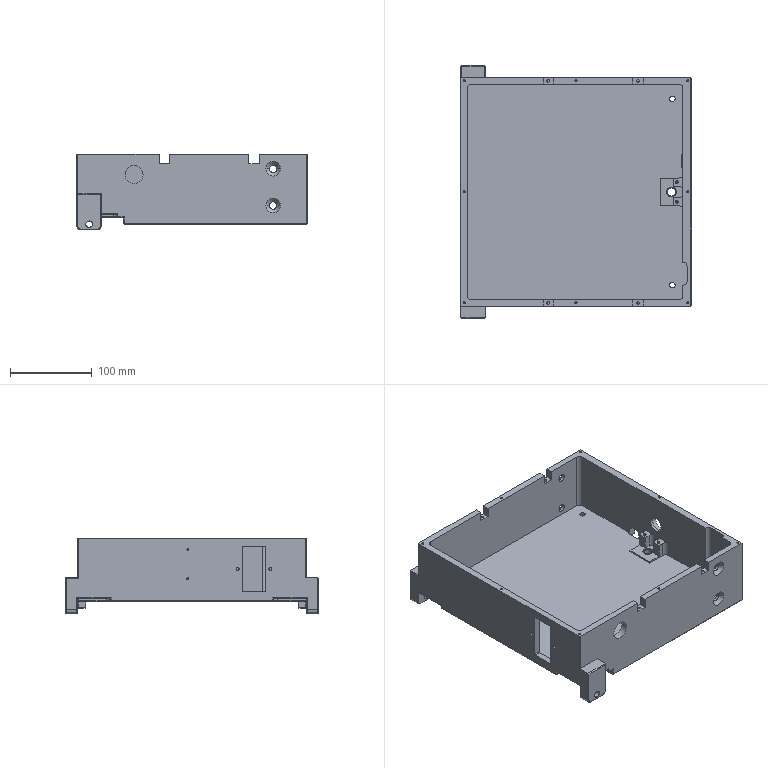NC program | Mastercam | posted with a generic post
Lines 36208 to 38289 of 104433, first 1964 of 2082 lines:
(10 FEM |TOOL - 10|DIA. OFF. - 10|LEN. - 10|TOOL DIA. - 10.)
N3176 T10 M6
N3178 G0 G54 G90 X-125. Y35.15 C0. B0. S7000 M3
N3180 G43 H10 Z50.
N3182 Z1.
N3184 G1 Z-.7 F600.
N3186 X-132. F3000.
N3188 X-140.
N3190 X-147.
N3192 Z-1.4 F600.
N3194 X-140. F3000.
N3196 X-132.
N3198 X-125.
N3200 Z-2.1 F600.
N3202 X-132. F3000.
N3204 X-140.
N3206 X-147.
N3208 Z-2.8 F600.
N3210 X-140. F3000.
N3212 X-132.
N3214 X-125.
N3216 Z-3.5 F600.
N3218 X-132. F3000.
N3220 X-140.
N3222 X-147.
N3224 Z-4.2 F600.
N3226 X-140. F3000.
N3228 X-132.
N3230 X-125.
N3232 Z-4.9 F600.
N3234 X-132. F3000.
N3236 X-140.
N3238 X-147.
N3240 Z-5.6 F600.
N3242 X-140. F3000.
N3244 X-132.
N3246 X-125.
N3248 Z-6.3 F600.
N3250 X-132. F3000.
N3252 X-140.
N3254 X-147.
N3256 Z-7. F600.
N3258 X-140. F3000.
N3260 X-132.
N3262 X-125.
N3264 Z-7.7 F600.
N3266 X-132. F3000.
N3268 X-140.
N3270 X-147.
N3272 Z-8.4 F600.
N3274 X-140. F3000.
N3276 X-132.
N3278 X-125.
N3280 Z-9.1 F600.
N3282 X-132. F3000.
N3284 X-140.
N3286 X-147.
N3288 Z-9.8 F600.
N3290 X-140. F3000.
N3292 X-132.
N3294 X-125.
N3296 Z-10.5 F600.
N3298 X-132. F3000.
N3300 X-140.
N3302 X-147.
N3304 Z-11.2 F600.
N3306 X-140. F3000.
N3308 X-132.
N3310 X-125.
N3312 Z-11.9 F600.
N3314 X-132. F3000.
N3316 X-140.
N3318 X-147.
N3320 G0 Z50.
N3322 Y32.85
N3324 Z1.
N3326 G1 Z-.7 F600.
N3328 X-140. F3000.
N3330 X-132.
N3332 X-125.
N3334 Z-1.4 F600.
N3336 X-132. F3000.
N3338 X-140.
N3340 X-147.
N3342 Z-2.1 F600.
N3344 X-140. F3000.
N3346 X-132.
N3348 X-125.
N3350 Z-2.8 F600.
N3352 X-132. F3000.
N3354 X-140.
N3356 X-147.
N3358 Z-3.5 F600.
N3360 X-140. F3000.
N3362 X-132.
N3364 X-125.
N3366 Z-4.2 F600.
N3368 X-132. F3000.
N3370 X-140.
N3372 X-147.
N3374 Z-4.9 F600.
N3376 X-140. F3000.
N3378 X-132.
N3380 X-125.
N3382 Z-5.6 F600.
N3384 X-132. F3000.
N3386 X-140.
N3388 X-147.
N3390 Z-6.3 F600.
N3392 X-140. F3000.
N3394 X-132.
N3396 X-125.
N3398 Z-7. F600.
N3400 X-132. F3000.
N3402 X-140.
N3404 X-147.
N3406 Z-7.7 F600.
N3408 X-140. F3000.
N3410 X-132.
N3412 X-125.
N3414 Z-8.4 F600.
N3416 X-132. F3000.
N3418 X-140.
N3420 X-147.
N3422 Z-9.1 F600.
N3424 X-140. F3000.
N3426 X-132.
N3428 X-125.
N3430 Z-9.8 F600.
N3432 X-132. F3000.
N3434 X-140.
N3436 X-147.
N3438 Z-10.5 F600.
N3440 X-140. F3000.
N3442 X-132.
N3444 X-125.
N3446 Z-11.2 F600.
N3448 X-132. F3000.
N3450 X-140.
N3452 X-147.
N3454 Z-11.9 F600.
N3456 X-140. F3000.
N3458 X-132.
N3460 X-125.
N3462 G0 Z50.
N3464 Y-74.85
N3466 Z1.
N3468 G1 Z-.7 F600.
N3470 X-132. F3000.
N3472 X-140.
N3474 X-147.
N3476 Z-1.4 F600.
N3478 X-140. F3000.
N3480 X-132.
N3482 X-125.
N3484 Z-2.1 F600.
N3486 X-132. F3000.
N3488 X-140.
N3490 X-147.
N3492 Z-2.8 F600.
N3494 X-140. F3000.
N3496 X-132.
N3498 X-125.
N3500 Z-3.5 F600.
N3502 X-132. F3000.
N3504 X-140.
N3506 X-147.
N3508 Z-4.2 F600.
N3510 X-140. F3000.
N3512 X-132.
N3514 X-125.
N3516 Z-4.9 F600.
N3518 X-132. F3000.
N3520 X-140.
N3522 X-147.
N3524 Z-5.6 F600.
N3526 X-140. F3000.
N3528 X-132.
N3530 X-125.
N3532 Z-6.3 F600.
N3534 X-132. F3000.
N3536 X-140.
N3538 X-147.
N3540 Z-7. F600.
N3542 X-140. F3000.
N3544 X-132.
N3546 X-125.
N3548 Z-7.7 F600.
N3550 X-132. F3000.
N3552 X-140.
N3554 X-147.
N3556 Z-8.4 F600.
N3558 X-140. F3000.
N3560 X-132.
N3562 X-125.
N3564 Z-9.1 F600.
N3566 X-132. F3000.
N3568 X-140.
N3570 X-147.
N3572 Z-9.8 F600.
N3574 X-140. F3000.
N3576 X-132.
N3578 X-125.
N3580 Z-10.5 F600.
N3582 X-132. F3000.
N3584 X-140.
N3586 X-147.
N3588 Z-11.2 F600.
N3590 X-140. F3000.
N3592 X-132.
N3594 X-125.
N3596 Z-11.9 F600.
N3598 X-132. F3000.
N3600 X-140.
N3602 X-147.
N3604 G0 Z50.
N3606 Y-77.15
N3608 Z1.
N3610 G1 Z-.7 F600.
N3612 X-140. F3000.
N3614 X-132.
N3616 X-125.
N3618 Z-1.4 F600.
N3620 X-132. F3000.
N3622 X-140.
N3624 X-147.
N3626 Z-2.1 F600.
N3628 X-140. F3000.
N3630 X-132.
N3632 X-125.
N3634 Z-2.8 F600.
N3636 X-132. F3000.
N3638 X-140.
N3640 X-147.
N3642 Z-3.5 F600.
N3644 X-140. F3000.
N3646 X-132.
N3648 X-125.
N3650 Z-4.2 F600.
N3652 X-132. F3000.
N3654 X-140.
N3656 X-147.
N3658 Z-4.9 F600.
N3660 X-140. F3000.
N3662 X-132.
N3664 X-125.
N3666 Z-5.6 F600.
N3668 X-132. F3000.
N3670 X-140.
N3672 X-147.
N3674 Z-6.3 F600.
N3676 X-140. F3000.
N3678 X-132.
N3680 X-125.
N3682 Z-7. F600.
N3684 X-132. F3000.
N3686 X-140.
N3688 X-147.
N3690 Z-7.7 F600.
N3692 X-140. F3000.
N3694 X-132.
N3696 X-125.
N3698 Z-8.4 F600.
N3700 X-132. F3000.
N3702 X-140.
N3704 X-147.
N3706 Z-9.1 F600.
N3708 X-140. F3000.
N3710 X-132.
N3712 X-125.
N3714 Z-9.8 F600.
N3716 X-132. F3000.
N3718 X-140.
N3720 X-147.
N3722 Z-10.5 F600.
N3724 X-140. F3000.
N3726 X-132.
N3728 X-125.
N3730 Z-11.2 F600.
N3732 X-132. F3000.
N3734 X-140.
N3736 X-147.
N3738 Z-11.9 F600.
N3740 X-140. F3000.
N3742 X-132.
N3744 X-125.
N3746 G0 Z50.
N3748 X147. Y-74.85
N3750 Z1.
N3752 G1 Z-.7 F600.
N3754 X140. F3000.
N3756 X132.
N3758 X125.
N3760 Z-1.4 F600.
N3762 X132. F3000.
N3764 X140.
N3766 X147.
N3768 Z-2.1 F600.
N3770 X140. F3000.
N3772 X132.
N3774 X125.
N3776 Z-2.8 F600.
N3778 X132. F3000.
N3780 X140.
N3782 X147.
N3784 Z-3.5 F600.
N3786 X140. F3000.
N3788 X132.
N3790 X125.
N3792 Z-4.2 F600.
N3794 X132. F3000.
N3796 X140.
N3798 X147.
N3800 Z-4.9 F600.
N3802 X140. F3000.
N3804 X132.
N3806 X125.
N3808 Z-5.6 F600.
N3810 X132. F3000.
N3812 X140.
N3814 X147.
N3816 Z-6.3 F600.
N3818 X140. F3000.
N3820 X132.
N3822 X125.
N3824 Z-7. F600.
N3826 X132. F3000.
N3828 X140.
N3830 X147.
N3832 Z-7.7 F600.
N3834 X140. F3000.
N3836 X132.
N3838 X125.
N3840 Z-8.4 F600.
N3842 X132. F3000.
N3844 X140.
N3846 X147.
N3848 Z-9.1 F600.
N3850 X140. F3000.
N3852 X132.
N3854 X125.
N3856 Z-9.8 F600.
N3858 X132. F3000.
N3860 X140.
N3862 X147.
N3864 Z-10.5 F600.
N3866 X140. F3000.
N3868 X132.
N3870 X125.
N3872 Z-11.2 F600.
N3874 X132. F3000.
N3876 X140.
N3878 X147.
N3880 Z-11.9 F600.
N3882 X140. F3000.
N3884 X132.
N3886 X125.
N3888 G0 Z50.
N3890 Y-77.15
N3892 Z1.
N3894 G1 Z-.7 F600.
N3896 X132. F3000.
N3898 X140.
N3900 X147.
N3902 Z-1.4 F600.
N3904 X140. F3000.
N3906 X132.
N3908 X125.
N3910 Z-2.1 F600.
N3912 X132. F3000.
N3914 X140.
N3916 X147.
N3918 Z-2.8 F600.
N3920 X140. F3000.
N3922 X132.
N3924 X125.
N3926 Z-3.5 F600.
N3928 X132. F3000.
N3930 X140.
N3932 X147.
N3934 Z-4.2 F600.
N3936 X140. F3000.
N3938 X132.
N3940 X125.
N3942 Z-4.9 F600.
N3944 X132. F3000.
N3946 X140.
N3948 X147.
N3950 Z-5.6 F600.
N3952 X140. F3000.
N3954 X132.
N3956 X125.
N3958 Z-6.3 F600.
N3960 X132. F3000.
N3962 X140.
N3964 X147.
N3966 Z-7. F600.
N3968 X140. F3000.
N3970 X132.
N3972 X125.
N3974 Z-7.7 F600.
N3976 X132. F3000.
N3978 X140.
N3980 X147.
N3982 Z-8.4 F600.
N3984 X140. F3000.
N3986 X132.
N3988 X125.
N3990 Z-9.1 F600.
N3992 X132. F3000.
N3994 X140.
N3996 X147.
N3998 Z-9.8 F600.
N4000 X140. F3000.
N4002 X132.
N4004 X125.
N4006 Z-10.5 F600.
N4008 X132. F3000.
N4010 X140.
N4012 X147.
N4014 Z-11.2 F600.
N4016 X140. F3000.
N4018 X132.
N4020 X125.
N4022 Z-11.9 F600.
N4024 X132. F3000.
N4026 X140.
N4028 X147.
N4030 G0 Z50.
N4032 Y35.15
N4034 Z1.
N4036 G1 Z-.7 F600.
N4038 X140. F3000.
N4040 X132.
N4042 X125.
N4044 Z-1.4 F600.
N4046 X132. F3000.
N4048 X140.
N4050 X147.
N4052 Z-2.1 F600.
N4054 X140. F3000.
N4056 X132.
N4058 X125.
N4060 Z-2.8 F600.
N4062 X132. F3000.
N4064 X140.
N4066 X147.
N4068 Z-3.5 F600.
N4070 X140. F3000.
N4072 X132.
N4074 X125.
N4076 Z-4.2 F600.
N4078 X132. F3000.
N4080 X140.
N4082 X147.
N4084 Z-4.9 F600.
N4086 X140. F3000.
N4088 X132.
N4090 X125.
N4092 Z-5.6 F600.
N4094 X132. F3000.
N4096 X140.
N4098 X147.
N4100 Z-6.3 F600.
N4102 X140. F3000.
N4104 X132.
N4106 X125.
N4108 Z-7. F600.
N4110 X132. F3000.
N4112 X140.
N4114 X147.
N4116 Z-7.7 F600.
N4118 X140. F3000.
N4120 X132.
N4122 X125.
N4124 Z-8.4 F600.
N4126 X132. F3000.
N4128 X140.
N4130 X147.
N4132 Z-9.1 F600.
N4134 X140. F3000.
N4136 X132.
N4138 X125.
N4140 Z-9.8 F600.
N4142 X132. F3000.
N4144 X140.
N4146 X147.
N4148 Z-10.5 F600.
N4150 X140. F3000.
N4152 X132.
N4154 X125.
N4156 Z-11.2 F600.
N4158 X132. F3000.
N4160 X140.
N4162 X147.
N4164 Z-11.9 F600.
N4166 X140. F3000.
N4168 X132.
N4170 X125.
N4172 G0 Z50.
N4174 Y32.85
N4176 Z1.
N4178 G1 Z-.7 F600.
N4180 X132. F3000.
N4182 X140.
N4184 X147.
N4186 Z-1.4 F600.
N4188 X140. F3000.
N4190 X132.
N4192 X125.
N4194 Z-2.1 F600.
N4196 X132. F3000.
N4198 X140.
N4200 X147.
N4202 Z-2.8 F600.
N4204 X140. F3000.
N4206 X132.
N4208 X125.
N4210 Z-3.5 F600.
N4212 X132. F3000.
N4214 X140.
N4216 X147.
N4218 Z-4.2 F600.
N4220 X140. F3000.
N4222 X132.
N4224 X125.
N4226 Z-4.9 F600.
N4228 X132. F3000.
N4230 X140.
N4232 X147.
N4234 Z-5.6 F600.
N4236 X140. F3000.
N4238 X132.
N4240 X125.
N4242 Z-6.3 F600.
N4244 X132. F3000.
N4246 X140.
N4248 X147.
N4250 Z-7. F600.
N4252 X140. F3000.
N4254 X132.
N4256 X125.
N4258 Z-7.7 F600.
N4260 X132. F3000.
N4262 X140.
N4264 X147.
N4266 Z-8.4 F600.
N4268 X140. F3000.
N4270 X132.
N4272 X125.
N4274 Z-9.1 F600.
N4276 X132. F3000.
N4278 X140.
N4280 X147.
N4282 Z-9.8 F600.
N4284 X140. F3000.
N4286 X132.
N4288 X125.
N4290 Z-10.5 F600.
N4292 X132. F3000.
N4294 X140.
N4296 X147.
N4298 Z-11.2 F600.
N4300 X140. F3000.
N4302 X132.
N4304 X125.
N4306 Z-11.9 F600.
N4308 X132. F3000.
N4310 X140.
N4312 X147.
N4314 G0 Z50.
N4316 X-125. Y35.26
N4318 Z1.
N4320 G1 Z-12. F600.
N4322 X-132. F1000.
N4324 X-140.
N4326 X-147.
N4328 G0 Z50.
N4330 Y32.74
N4332 Z1.
N4334 G1 Z-12. F600.
N4336 X-140. F1000.
N4338 X-132.
N4340 X-125.
N4342 G0 Z50.
N4344 Y-74.74
N4346 Z1.
N4348 G1 Z-12. F600.
N4350 X-132. F1000.
N4352 X-140.
N4354 X-147.
N4356 G0 Z50.
N4358 Y-77.26
N4360 Z1.
N4362 G1 Z-12. F600.
N4364 X-140. F1000.
N4366 X-132.
N4368 X-125.
N4370 G0 Z50.
N4372 X147. Y-74.74
N4374 Z1.
N4376 G1 Z-12. F600.
N4378 X140. F1000.
N4380 X132.
N4382 X125.
N4384 G0 Z50.
N4386 Y-77.26
N4388 Z1.
N4390 G1 Z-12. F600.
N4392 X132. F1000.
N4394 X140.
N4396 X147.
N4398 G0 Z50.
N4400 Y35.26
N4402 Z1.
N4404 G1 Z-12. F600.
N4406 X140. F1000.
N4408 X132.
N4410 X125.
N4412 G0 Z50.
N4414 Y32.74
N4416 Z1.
N4418 G1 Z-12. F600.
N4420 X132. F1000.
N4422 X140.
N4424 X147.
N4426 G0 Z50.
N4428 M5
N4430 G0 G28 G91 Z0.
N4432 G28
N4434 M01
N4436 G0 G17 G40 G80 G90 G94 G98
N4438 G0 G28 G91 Z0.
(20 FEM |TOOL - 20|DIA. OFF. - 20|LEN. - 20|TOOL DIA. - 20.)
N4440 T20 M6
N4442 G0 G54 G90 X155.627 Y-138.656 C0. B0. S4000 M3
N4444 G43 H20 Z50.
N4446 Z1.
N4448 G1 Z-24. F600.
N4450 X147.142 Y-147.142 F2000.
N4452 X146.142 Y-148.142
N4454 G2 X139. Y-151.1 I-7.142 J7.142
N4456 G1 X-139.
N4458 G2 X-146.142 Y-148.142 J10.1
N4460 G1 X-147.142 Y-147.142
N4462 G2 X-150.1 Y-140. I7.142 J7.142
N4464 G1 Y140.
N4466 G2 X-147.142 Y147.142 I10.1
N4468 G1 X-146.142 Y148.142
N4470 G2 X-139. Y151.1 I7.142 J-7.142
N4472 G1 X139.
N4474 G2 X146.142 Y148.142 J-10.1
N4476 G1 X147.142 Y147.142
N4478 G2 X150.1 Y140. I-7.142 J-7.142
N4480 G1 Y-140.
N4482 G2 X147.142 Y-147.142 I-10.1
N4484 G1 X146.788 Y-147.495
N4486 X137.596 Y-156.688
N4488 G0 Z50.
N4490 X155.556 Y-138.586
N4492 Z1.
N4494 G1 Z-24. F600.
N4496 X147.071 Y-147.071 F2000.
N4498 X146.071 Y-148.071
N4500 G2 X139. Y-151. I-7.071 J7.071
N4502 G1 X-139.
N4504 G2 X-146.071 Y-148.071 J10.
N4506 G1 X-147.071 Y-147.071
N4508 G2 X-150. Y-140. I7.071 J7.071
N4510 G1 Y140.
N4512 G2 X-147.071 Y147.071 I10.
N4514 G1 X-146.071 Y148.071
N4516 G2 X-139. Y151. I7.071 J-7.071
N4518 G1 X139.
N4520 G2 X146.071 Y148.071 J-10.
N4522 G1 X147.071 Y147.071
N4524 G2 X150. Y140. I-7.071 J-7.071
N4526 G1 Y-140.
N4528 G2 X147.071 Y-147.071 I-10.
N4530 G1 X146.718 Y-147.425
N4532 X137.525 Y-156.617
N4534 G0 Z50.
N4536 X155.627 Y-138.656
N4538 Z-23.
N4540 G1 Z-48. F600.
N4542 X147.142 Y-147.142 F2000.
N4544 X146.142 Y-148.142
N4546 G2 X139. Y-151.1 I-7.142 J7.142
N4548 G1 X-139.
N4550 G2 X-146.142 Y-148.142 J10.1
N4552 G1 X-147.142 Y-147.142
N4554 G2 X-150.1 Y-140. I7.142 J7.142
N4556 G1 Y140.
N4558 G2 X-147.142 Y147.142 I10.1
N4560 G1 X-146.142 Y148.142
N4562 G2 X-139. Y151.1 I7.142 J-7.142
N4564 G1 X139.
N4566 G2 X146.142 Y148.142 J-10.1
N4568 G1 X147.142 Y147.142
N4570 G2 X150.1 Y140. I-7.142 J-7.142
N4572 G1 Y-140.
N4574 G2 X147.142 Y-147.142 I-10.1
N4576 G1 X146.788 Y-147.495
N4578 X137.596 Y-156.688
N4580 G0 Z50.
N4582 X155.556 Y-138.586
N4584 Z-23.
N4586 G1 Z-48. F600.
N4588 X147.071 Y-147.071 F2000.
N4590 X146.071 Y-148.071
N4592 G2 X139. Y-151. I-7.071 J7.071
N4594 G1 X-139.
N4596 G2 X-146.071 Y-148.071 J10.
N4598 G1 X-147.071 Y-147.071
N4600 G2 X-150. Y-140. I7.071 J7.071
N4602 G1 Y140.
N4604 G2 X-147.071 Y147.071 I10.
N4606 G1 X-146.071 Y148.071
N4608 G2 X-139. Y151. I7.071 J-7.071
N4610 G1 X139.
N4612 G2 X146.071 Y148.071 J-10.
N4614 G1 X147.071 Y147.071
N4616 G2 X150. Y140. I-7.071 J-7.071
N4618 G1 Y-140.
N4620 G2 X147.071 Y-147.071 I-10.
N4622 G1 X146.718 Y-147.425
N4624 X137.525 Y-156.617
N4626 G0 Z50.
N4628 X-154.1 Y82.619
N4630 Z-47.
N4632 G1 Z-48.989 F600.
N4634 X-152.1 F4000.
N4636 G3 X-150.1 Y84.619 J2.
N4638 G1 Y100.
N4640 G3 X-151. Y100.9 I-.9
N4642 G1 X-154.
N4644 G2 X-161.142 Y103.858 J10.1
N4646 G1 X-162.142 Y104.858
N4648 G2 X-165.1 Y112. I7.142 J7.142
N4650 G1 Y114.316
N4652 G3 X-167.1 Y116.316 I-2.
N4654 G1 X-169.1
N4656 X-154.1 Y82.619
N4658 Z-49.978 F600.
N4660 X-152.1 F4000.
N4662 G3 X-150.1 Y84.619 J2.
N4664 G1 Y100.
N4666 G3 X-151. Y100.9 I-.9
N4668 G1 X-154.
N4670 G2 X-161.142 Y103.858 J10.1
N4672 G1 X-162.142 Y104.858
N4674 G2 X-165.1 Y112. I7.142 J7.142
N4676 G1 Y114.316
N4678 G3 X-167.1 Y116.316 I-2.
N4680 G1 X-169.1
N4682 X-154.1 Y82.619
N4684 Z-50.967 F600.
N4686 X-152.1 F4000.
N4688 G3 X-150.1 Y84.619 J2.
N4690 G1 Y100.
N4692 G3 X-151. Y100.9 I-.9
N4694 G1 X-154.
N4696 G2 X-161.142 Y103.858 J10.1
N4698 G1 X-162.142 Y104.858
N4700 G2 X-165.1 Y112. I7.142 J7.142
N4702 G1 Y114.316
N4704 G3 X-167.1 Y116.316 I-2.
N4706 G1 X-169.1
N4708 X-154.1 Y82.619
N4710 Z-51.957 F600.
N4712 X-152.1 F4000.
N4714 G3 X-150.1 Y84.619 J2.
N4716 G1 Y100.
N4718 G3 X-151. Y100.9 I-.9
N4720 G1 X-154.
N4722 G2 X-161.142 Y103.858 J10.1
N4724 G1 X-162.142 Y104.858
N4726 G2 X-165.1 Y112. I7.142 J7.142
N4728 G1 Y114.316
N4730 G3 X-167.1 Y116.316 I-2.
N4732 G1 X-169.1
N4734 X-154.1 Y82.619
N4736 Z-52.946 F600.
N4738 X-152.1 F4000.
N4740 G3 X-150.1 Y84.619 J2.
N4742 G1 Y100.
N4744 G3 X-151. Y100.9 I-.9
N4746 G1 X-154.
N4748 G2 X-161.142 Y103.858 J10.1
N4750 G1 X-162.142 Y104.858
N4752 G2 X-165.1 Y112. I7.142 J7.142
N4754 G1 Y114.316
N4756 G3 X-167.1 Y116.316 I-2.
N4758 G1 X-169.1
N4760 X-154.1 Y82.619
N4762 Z-53.935 F600.
N4764 X-152.1 F4000.
N4766 G3 X-150.1 Y84.619 J2.
N4768 G1 Y100.
N4770 G3 X-151. Y100.9 I-.9
N4772 G1 X-154.
N4774 G2 X-161.142 Y103.858 J10.1
N4776 G1 X-162.142 Y104.858
N4778 G2 X-165.1 Y112. I7.142 J7.142
N4780 G1 Y114.316
N4782 G3 X-167.1 Y116.316 I-2.
N4784 G1 X-169.1
N4786 X-154.1 Y82.619
N4788 Z-54.924 F600.
N4790 X-152.1 F4000.
N4792 G3 X-150.1 Y84.619 J2.
N4794 G1 Y100.
N4796 G3 X-151. Y100.9 I-.9
N4798 G1 X-154.
N4800 G2 X-161.142 Y103.858 J10.1
N4802 G1 X-162.142 Y104.858
N4804 G2 X-165.1 Y112. I7.142 J7.142
N4806 G1 Y114.316
N4808 G3 X-167.1 Y116.316 I-2.
N4810 G1 X-169.1
N4812 X-154.1 Y82.619
N4814 Z-55.913 F600.
N4816 X-152.1 F4000.
N4818 G3 X-150.1 Y84.619 J2.
N4820 G1 Y100.
N4822 G3 X-151. Y100.9 I-.9
N4824 G1 X-154.
N4826 G2 X-161.142 Y103.858 J10.1
N4828 G1 X-162.142 Y104.858
N4830 G2 X-165.1 Y112. I7.142 J7.142
N4832 G1 Y114.316
N4834 G3 X-167.1 Y116.316 I-2.
N4836 G1 X-169.1
N4838 X-154.1 Y82.619
N4840 Z-56.902 F600.
N4842 X-152.1 F4000.
N4844 G3 X-150.1 Y84.619 J2.
N4846 G1 Y100.
N4848 G3 X-151. Y100.9 I-.9
N4850 G1 X-154.
N4852 G2 X-161.142 Y103.858 J10.1
N4854 G1 X-162.142 Y104.858
N4856 G2 X-165.1 Y112. I7.142 J7.142
N4858 G1 Y114.316
N4860 G3 X-167.1 Y116.316 I-2.
N4862 G1 X-169.1
N4864 X-154.1 Y82.619
N4866 Z-57.891 F600.
N4868 X-152.1 F4000.
N4870 G3 X-150.1 Y84.619 J2.
N4872 G1 Y100.
N4874 G3 X-151. Y100.9 I-.9
N4876 G1 X-154.
N4878 G2 X-161.142 Y103.858 J10.1
N4880 G1 X-162.142 Y104.858
N4882 G2 X-165.1 Y112. I7.142 J7.142
N4884 G1 Y114.316
N4886 G3 X-167.1 Y116.316 I-2.
N4888 G1 X-169.1
N4890 X-154.1 Y82.619
N4892 Z-58.88 F600.
N4894 X-152.1 F4000.
N4896 G3 X-150.1 Y84.619 J2.
N4898 G1 Y100.
N4900 G3 X-151. Y100.9 I-.9
N4902 G1 X-154.
N4904 G2 X-161.142 Y103.858 J10.1
N4906 G1 X-162.142 Y104.858
N4908 G2 X-165.1 Y112. I7.142 J7.142
N4910 G1 Y114.316
N4912 G3 X-167.1 Y116.316 I-2.
N4914 G1 X-169.1
N4916 X-154.1 Y82.619
N4918 Z-59.87 F600.
N4920 X-152.1 F4000.
N4922 G3 X-150.1 Y84.619 J2.
N4924 G1 Y100.
N4926 G3 X-151. Y100.9 I-.9
N4928 G1 X-154.
N4930 G2 X-161.142 Y103.858 J10.1
N4932 G1 X-162.142 Y104.858
N4934 G2 X-165.1 Y112. I7.142 J7.142
N4936 G1 Y114.316
N4938 G3 X-167.1 Y116.316 I-2.
N4940 G1 X-169.1
N4942 X-154.1 Y82.619
N4944 Z-60.859 F600.
N4946 X-152.1 F4000.
N4948 G3 X-150.1 Y84.619 J2.
N4950 G1 Y100.
N4952 G3 X-151. Y100.9 I-.9
N4954 G1 X-154.
N4956 G2 X-161.142 Y103.858 J10.1
N4958 G1 X-162.142 Y104.858
N4960 G2 X-165.1 Y112. I7.142 J7.142
N4962 G1 Y114.316
N4964 G3 X-167.1 Y116.316 I-2.
N4966 G1 X-169.1
N4968 X-154.1 Y82.619
N4970 Z-61.848 F600.
N4972 X-152.1 F4000.
N4974 G3 X-150.1 Y84.619 J2.
N4976 G1 Y100.
N4978 G3 X-151. Y100.9 I-.9
N4980 G1 X-154.
N4982 G2 X-161.142 Y103.858 J10.1
N4984 G1 X-162.142 Y104.858
N4986 G2 X-165.1 Y112. I7.142 J7.142
N4988 G1 Y114.316
N4990 G3 X-167.1 Y116.316 I-2.
N4992 G1 X-169.1
N4994 X-154.1 Y82.619
N4996 Z-62.837 F600.
N4998 X-152.1 F4000.
N5000 G3 X-150.1 Y84.619 J2.
N5002 G1 Y100.
N5004 G3 X-151. Y100.9 I-.9
N5006 G1 X-154.
N5008 G2 X-161.142 Y103.858 J10.1
N5010 G1 X-162.142 Y104.858
N5012 G2 X-165.1 Y112. I7.142 J7.142
N5014 G1 Y114.316
N5016 G3 X-167.1 Y116.316 I-2.
N5018 G1 X-169.1
N5020 X-154.1 Y82.619
N5022 Z-63.826 F600.
N5024 X-152.1 F4000.
N5026 G3 X-150.1 Y84.619 J2.
N5028 G1 Y100.
N5030 G3 X-151. Y100.9 I-.9
N5032 G1 X-154.
N5034 G2 X-161.142 Y103.858 J10.1
N5036 G1 X-162.142 Y104.858
N5038 G2 X-165.1 Y112. I7.142 J7.142
N5040 G1 Y114.316
N5042 G3 X-167.1 Y116.316 I-2.
N5044 G1 X-169.1
N5046 X-154.1 Y82.619
N5048 Z-64.815 F600.
N5050 X-152.1 F4000.
N5052 G3 X-150.1 Y84.619 J2.
N5054 G1 Y100.
N5056 G3 X-151. Y100.9 I-.9
N5058 G1 X-154.
N5060 G2 X-161.142 Y103.858 J10.1
N5062 G1 X-162.142 Y104.858
N5064 G2 X-165.1 Y112. I7.142 J7.142
N5066 G1 Y114.316
N5068 G3 X-167.1 Y116.316 I-2.
N5070 G1 X-169.1
N5072 X-154.1 Y82.619
N5074 Z-65.804 F600.
N5076 X-152.1 F4000.
N5078 G3 X-150.1 Y84.619 J2.
N5080 G1 Y100.
N5082 G3 X-151. Y100.9 I-.9
N5084 G1 X-154.
N5086 G2 X-161.142 Y103.858 J10.1
N5088 G1 X-162.142 Y104.858
N5090 G2 X-165.1 Y112. I7.142 J7.142
N5092 G1 Y114.316
N5094 G3 X-167.1 Y116.316 I-2.
N5096 G1 X-169.1
N5098 X-154.1 Y82.619
N5100 Z-66.793 F600.
N5102 X-152.1 F4000.
N5104 G3 X-150.1 Y84.619 J2.
N5106 G1 Y100.
N5108 G3 X-151. Y100.9 I-.9
N5110 G1 X-154.
N5112 G2 X-161.142 Y103.858 J10.1
N5114 G1 X-162.142 Y104.858
N5116 G2 X-165.1 Y112. I7.142 J7.142
N5118 G1 Y114.316
N5120 G3 X-167.1 Y116.316 I-2.
N5122 G1 X-169.1
N5124 X-154.1 Y82.619
N5126 Z-67.783 F600.
N5128 X-152.1 F4000.
N5130 G3 X-150.1 Y84.619 J2.
N5132 G1 Y100.
N5134 G3 X-151. Y100.9 I-.9
N5136 G1 X-154.
N5138 G2 X-161.142 Y103.858 J10.1
N5140 G1 X-162.142 Y104.858
N5142 G2 X-165.1 Y112. I7.142 J7.142
N5144 G1 Y114.316
N5146 G3 X-167.1 Y116.316 I-2.
N5148 G1 X-169.1
N5150 X-154.1 Y82.619
N5152 Z-68.772 F600.
N5154 X-152.1 F4000.
N5156 G3 X-150.1 Y84.619 J2.
N5158 G1 Y100.
N5160 G3 X-151. Y100.9 I-.9
N5162 G1 X-154.
N5164 G2 X-161.142 Y103.858 J10.1
N5166 G1 X-162.142 Y104.858
N5168 G2 X-165.1 Y112. I7.142 J7.142
N5170 G1 Y114.316
N5172 G3 X-167.1 Y116.316 I-2.
N5174 G1 X-169.1
N5176 X-154.1 Y82.619
N5178 Z-69.761 F600.
N5180 X-152.1 F4000.
N5182 G3 X-150.1 Y84.619 J2.
N5184 G1 Y100.
N5186 G3 X-151. Y100.9 I-.9
N5188 G1 X-154.
N5190 G2 X-161.142 Y103.858 J10.1
N5192 G1 X-162.142 Y104.858
N5194 G2 X-165.1 Y112. I7.142 J7.142
N5196 G1 Y114.316
N5198 G3 X-167.1 Y116.316 I-2.
N5200 G1 X-169.1
N5202 X-154.1 Y82.619
N5204 Z-70.75 F600.
N5206 X-152.1 F4000.
N5208 G3 X-150.1 Y84.619 J2.
N5210 G1 Y100.
N5212 G3 X-151. Y100.9 I-.9
N5214 G1 X-154.
N5216 G2 X-161.142 Y103.858 J10.1
N5218 G1 X-162.142 Y104.858
N5220 G2 X-165.1 Y112. I7.142 J7.142
N5222 G1 Y114.316
N5224 G3 X-167.1 Y116.316 I-2.
N5226 G1 X-169.1
N5228 X-154.1 Y82.619
N5230 Z-71.739 F600.
N5232 X-152.1 F4000.
N5234 G3 X-150.1 Y84.619 J2.
N5236 G1 Y100.
N5238 G3 X-151. Y100.9 I-.9
N5240 G1 X-154.
N5242 G2 X-161.142 Y103.858 J10.1
N5244 G1 X-162.142 Y104.858
N5246 G2 X-165.1 Y112. I7.142 J7.142
N5248 G1 Y114.316
N5250 G3 X-167.1 Y116.316 I-2.
N5252 G1 X-169.1
N5254 X-154.1 Y82.619
N5256 Z-72.728 F600.
N5258 X-152.1 F4000.
N5260 G3 X-150.1 Y84.619 J2.
N5262 G1 Y100.
N5264 G3 X-151. Y100.9 I-.9
N5266 G1 X-154.
N5268 G2 X-161.142 Y103.858 J10.1
N5270 G1 X-162.142 Y104.858
N5272 G2 X-165.1 Y112. I7.142 J7.142
N5274 G1 Y114.316
N5276 G3 X-167.1 Y116.316 I-2.
N5278 G1 X-169.1
N5280 X-154.1 Y82.619
N5282 Z-73.717 F600.
N5284 X-152.1 F4000.
N5286 G3 X-150.1 Y84.619 J2.
N5288 G1 Y100.
N5290 G3 X-151. Y100.9 I-.9
N5292 G1 X-154.
N5294 G2 X-161.142 Y103.858 J10.1
N5296 G1 X-162.142 Y104.858
N5298 G2 X-165.1 Y112. I7.142 J7.142
N5300 G1 Y114.316
N5302 G3 X-167.1 Y116.316 I-2.
N5304 G1 X-169.1
N5306 X-154.1 Y82.619
N5308 Z-74.707 F600.
N5310 X-152.1 F4000.
N5312 G3 X-150.1 Y84.619 J2.
N5314 G1 Y100.
N5316 G3 X-151. Y100.9 I-.9
N5318 G1 X-154.
N5320 G2 X-161.142 Y103.858 J10.1
N5322 G1 X-162.142 Y104.858
N5324 G2 X-165.1 Y112. I7.142 J7.142
N5326 G1 Y114.316
N5328 G3 X-167.1 Y116.316 I-2.
N5330 G1 X-169.1
N5332 X-154.1 Y82.619
N5334 Z-75.696 F600.
N5336 X-152.1 F4000.
N5338 G3 X-150.1 Y84.619 J2.
N5340 G1 Y100.
N5342 G3 X-151. Y100.9 I-.9
N5344 G1 X-154.
N5346 G2 X-161.142 Y103.858 J10.1
N5348 G1 X-162.142 Y104.858
N5350 G2 X-165.1 Y112. I7.142 J7.142
N5352 G1 Y114.316
N5354 G3 X-167.1 Y116.316 I-2.
N5356 G1 X-169.1
N5358 X-154.1 Y82.619
N5360 Z-76.685 F600.
N5362 X-152.1 F4000.
N5364 G3 X-150.1 Y84.619 J2.
N5366 G1 Y100.
N5368 G3 X-151. Y100.9 I-.9
N5370 G1 X-154.
N5372 G2 X-161.142 Y103.858 J10.1
N5374 G1 X-162.142 Y104.858
N5376 G2 X-165.1 Y112. I7.142 J7.142
N5378 G1 Y114.316
N5380 G3 X-167.1 Y116.316 I-2.
N5382 G1 X-169.1
N5384 X-154.1 Y82.619
N5386 Z-77.674 F600.
N5388 X-152.1 F4000.
N5390 G3 X-150.1 Y84.619 J2.
N5392 G1 Y100.
N5394 G3 X-151. Y100.9 I-.9
N5396 G1 X-154.
N5398 G2 X-161.142 Y103.858 J10.1
N5400 G1 X-162.142 Y104.858
N5402 G2 X-165.1 Y112. I7.142 J7.142
N5404 G1 Y114.316
N5406 G3 X-167.1 Y116.316 I-2.
N5408 G1 X-169.1
N5410 X-154.1 Y82.619
N5412 Z-78.663 F600.
N5414 X-152.1 F4000.
N5416 G3 X-150.1 Y84.619 J2.
N5418 G1 Y100.
N5420 G3 X-151. Y100.9 I-.9
N5422 G1 X-154.
N5424 G2 X-161.142 Y103.858 J10.1
N5426 G1 X-162.142 Y104.858
N5428 G2 X-165.1 Y112. I7.142 J7.142
N5430 G1 Y114.316
N5432 G3 X-167.1 Y116.316 I-2.
N5434 G1 X-169.1
N5436 X-154.1 Y82.619
N5438 Z-79.652 F600.
N5440 X-152.1 F4000.
N5442 G3 X-150.1 Y84.619 J2.
N5444 G1 Y100.
N5446 G3 X-151. Y100.9 I-.9
N5448 G1 X-154.
N5450 G2 X-161.142 Y103.858 J10.1
N5452 G1 X-162.142 Y104.858
N5454 G2 X-165.1 Y112. I7.142 J7.142
N5456 G1 Y114.316
N5458 G3 X-167.1 Y116.316 I-2.
N5460 G1 X-169.1
N5462 X-154.1 Y82.619
N5464 Z-80.641 F600.
N5466 X-152.1 F4000.
N5468 G3 X-150.1 Y84.619 J2.
N5470 G1 Y100.
N5472 G3 X-151. Y100.9 I-.9
N5474 G1 X-154.
N5476 G2 X-161.142 Y103.858 J10.1
N5478 G1 X-162.142 Y104.858
N5480 G2 X-165.1 Y112. I7.142 J7.142
N5482 G1 Y114.316
N5484 G3 X-167.1 Y116.316 I-2.
N5486 G1 X-169.1
N5488 X-154.1 Y82.619
N5490 Z-81.63 F600.
N5492 X-152.1 F4000.
N5494 G3 X-150.1 Y84.619 J2.
N5496 G1 Y100.
N5498 G3 X-151. Y100.9 I-.9
N5500 G1 X-154.
N5502 G2 X-161.142 Y103.858 J10.1
N5504 G1 X-162.142 Y104.858
N5506 G2 X-165.1 Y112. I7.142 J7.142
N5508 G1 Y114.316
N5510 G3 X-167.1 Y116.316 I-2.
N5512 G1 X-169.1
N5514 X-154.1 Y82.619
N5516 Z-82.62 F600.
N5518 X-152.1 F4000.
N5520 G3 X-150.1 Y84.619 J2.
N5522 G1 Y100.
N5524 G3 X-151. Y100.9 I-.9
N5526 G1 X-154.
N5528 G2 X-161.142 Y103.858 J10.1
N5530 G1 X-162.142 Y104.858
N5532 G2 X-165.1 Y112. I7.142 J7.142
N5534 G1 Y114.316
N5536 G3 X-167.1 Y116.316 I-2.
N5538 G1 X-169.1
N5540 X-154.1 Y82.619
N5542 Z-83.609 F600.
N5544 X-152.1 F4000.
N5546 G3 X-150.1 Y84.619 J2.
N5548 G1 Y100.
N5550 G3 X-151. Y100.9 I-.9
N5552 G1 X-154.
N5554 G2 X-161.142 Y103.858 J10.1
N5556 G1 X-162.142 Y104.858
N5558 G2 X-165.1 Y112. I7.142 J7.142
N5560 G1 Y114.316
N5562 G3 X-167.1 Y116.316 I-2.
N5564 G1 X-169.1
N5566 X-154.1 Y82.619
N5568 Z-84.598 F600.
N5570 X-152.1 F4000.
N5572 G3 X-150.1 Y84.619 J2.
N5574 G1 Y100.
N5576 G3 X-151. Y100.9 I-.9
N5578 G1 X-154.
N5580 G2 X-161.142 Y103.858 J10.1
N5582 G1 X-162.142 Y104.858
N5584 G2 X-165.1 Y112. I7.142 J7.142
N5586 G1 Y114.316
N5588 G3 X-167.1 Y116.316 I-2.
N5590 G1 X-169.1
N5592 X-154.1 Y82.619
N5594 Z-85.587 F600.
N5596 X-152.1 F4000.
N5598 G3 X-150.1 Y84.619 J2.
N5600 G1 Y100.
N5602 G3 X-151. Y100.9 I-.9
N5604 G1 X-154.
N5606 G2 X-161.142 Y103.858 J10.1
N5608 G1 X-162.142 Y104.858
N5610 G2 X-165.1 Y112. I7.142 J7.142
N5612 G1 Y114.316
N5614 G3 X-167.1 Y116.316 I-2.
N5616 G1 X-169.1
N5618 X-154.1 Y82.619
N5620 Z-86.576 F600.
N5622 X-152.1 F4000.
N5624 G3 X-150.1 Y84.619 J2.
N5626 G1 Y100.
N5628 G3 X-151. Y100.9 I-.9
N5630 G1 X-154.
N5632 G2 X-161.142 Y103.858 J10.1
N5634 G1 X-162.142 Y104.858
N5636 G2 X-165.1 Y112. I7.142 J7.142
N5638 G1 Y114.316
N5640 G3 X-167.1 Y116.316 I-2.
N5642 G1 X-169.1
N5644 X-154.1 Y82.619
N5646 Z-87.565 F600.
N5648 X-152.1 F4000.
N5650 G3 X-150.1 Y84.619 J2.
N5652 G1 Y100.
N5654 G3 X-151. Y100.9 I-.9
N5656 G1 X-154.
N5658 G2 X-161.142 Y103.858 J10.1
N5660 G1 X-162.142 Y104.858
N5662 G2 X-165.1 Y112. I7.142 J7.142
N5664 G1 Y114.316
N5666 G3 X-167.1 Y116.316 I-2.
N5668 G1 X-169.1
N5670 X-154.1 Y82.619
N5672 Z-88.554 F600.
N5674 X-152.1 F4000.
N5676 G3 X-150.1 Y84.619 J2.
N5678 G1 Y100.
N5680 G3 X-151. Y100.9 I-.9
N5682 G1 X-154.
N5684 G2 X-161.142 Y103.858 J10.1
N5686 G1 X-162.142 Y104.858
N5688 G2 X-165.1 Y112. I7.142 J7.142
N5690 G1 Y114.316
N5692 G3 X-167.1 Y116.316 I-2.
N5694 G1 X-169.1
N5696 X-154.1 Y82.619
N5698 Z-89.543 F600.
N5700 X-152.1 F4000.
N5702 G3 X-150.1 Y84.619 J2.
N5704 G1 Y100.
N5706 G3 X-151. Y100.9 I-.9
N5708 G1 X-154.
N5710 G2 X-161.142 Y103.858 J10.1
N5712 G1 X-162.142 Y104.858
N5714 G2 X-165.1 Y112. I7.142 J7.142
N5716 G1 Y114.316
N5718 G3 X-167.1 Y116.316 I-2.
N5720 G1 X-169.1
N5722 X-154.1 Y82.619
N5724 Z-90.533 F600.
N5726 X-152.1 F4000.
N5728 G3 X-150.1 Y84.619 J2.
N5730 G1 Y100.
N5732 G3 X-151. Y100.9 I-.9
N5734 G1 X-154.
N5736 G2 X-161.142 Y103.858 J10.1
N5738 G1 X-162.142 Y104.858
N5740 G2 X-165.1 Y112. I7.142 J7.142
N5742 G1 Y114.316
N5744 G3 X-167.1 Y116.316 I-2.
N5746 G1 X-169.1
N5748 X-154.1 Y82.619
N5750 Z-91.522 F600.
N5752 X-152.1 F4000.
N5754 G3 X-150.1 Y84.619 J2.
N5756 G1 Y100.
N5758 G3 X-151. Y100.9 I-.9
N5760 G1 X-154.
N5762 G2 X-161.142 Y103.858 J10.1
N5764 G1 X-162.142 Y104.858
N5766 G2 X-165.1 Y112. I7.142 J7.142
N5768 G1 Y114.316
N5770 G3 X-167.1 Y116.316 I-2.
N5772 G1 X-169.1
N5774 X-154.1 Y82.619
N5776 Z-92.511 F600.
N5778 X-152.1 F4000.
N5780 G3 X-150.1 Y84.619 J2.
N5782 G1 Y100.
N5784 G3 X-151. Y100.9 I-.9
N5786 G1 X-154.
N5788 G2 X-161.142 Y103.858 J10.1
N5790 G1 X-162.142 Y104.858
N5792 G2 X-165.1 Y112. I7.142 J7.142
N5794 G1 Y114.316
N5796 G3 X-167.1 Y116.316 I-2.
N5798 G1 X-169.1
N5800 X-154.1 Y82.619
N5802 Z-93.5 F600.
N5804 X-152.1 F4000.
N5806 G3 X-150.1 Y84.619 J2.
N5808 G1 Y100.
N5810 G3 X-151. Y100.9 I-.9
N5812 G1 X-154.
N5814 G2 X-161.142 Y103.858 J10.1
N5816 G1 X-162.142 Y104.858
N5818 G2 X-165.1 Y112. I7.142 J7.142
N5820 G1 Y114.316
N5822 G3 X-167.1 Y116.316 I-2.
N5824 G1 X-169.1
N5826 G0 Z50.
N5828 X169.1 Y116.281
N5830 Z-47.
N5832 G1 Z-48.989 F600.
N5834 X167.1 F4000.
N5836 G3 X165.1 Y114.281 J-2.
N5838 G1 Y112.
N5840 G2 X162.142 Y104.858 I-10.1
N5842 G1 X161.142 Y103.858
N5844 G2 X154. Y100.9 I-7.142 J7.142
N5846 G1 X151.
N5848 G3 X150.1 Y100. J-.9
N5850 G1 Y84.599
N5852 G3 X152.1 Y82.599 I2.
N5854 G1 X154.1
N5856 X169.1 Y116.281
N5858 Z-49.978 F600.
N5860 X167.1 F4000.
N5862 G3 X165.1 Y114.281 J-2.
N5864 G1 Y112.
N5866 G2 X162.142 Y104.858 I-10.1
N5868 G1 X161.142 Y103.858
N5870 G2 X154. Y100.9 I-7.142 J7.142
N5872 G1 X151.
N5874 G3 X150.1 Y100. J-.9
N5876 G1 Y84.599
N5878 G3 X152.1 Y82.599 I2.
N5880 G1 X154.1
N5882 X169.1 Y116.281
N5884 Z-50.967 F600.
N5886 X167.1 F4000.
N5888 G3 X165.1 Y114.281 J-2.
N5890 G1 Y112.
N5892 G2 X162.142 Y104.858 I-10.1
N5894 G1 X161.142 Y103.858
N5896 G2 X154. Y100.9 I-7.142 J7.142
N5898 G1 X151.
N5900 G3 X150.1 Y100. J-.9
N5902 G1 Y84.599
N5904 G3 X152.1 Y82.599 I2.
N5906 G1 X154.1
N5908 X169.1 Y116.281
N5910 Z-51.957 F600.
N5912 X167.1 F4000.
N5914 G3 X165.1 Y114.281 J-2.
N5916 G1 Y112.
N5918 G2 X162.142 Y104.858 I-10.1
N5920 G1 X161.142 Y103.858
N5922 G2 X154. Y100.9 I-7.142 J7.142
N5924 G1 X151.
N5926 G3 X150.1 Y100. J-.9
N5928 G1 Y84.599
N5930 G3 X152.1 Y82.599 I2.
N5932 G1 X154.1
N5934 X169.1 Y116.281
N5936 Z-52.946 F600.
N5938 X167.1 F4000.
N5940 G3 X165.1 Y114.281 J-2.
N5942 G1 Y112.
N5944 G2 X162.142 Y104.858 I-10.1
N5946 G1 X161.142 Y103.858
N5948 G2 X154. Y100.9 I-7.142 J7.142
N5950 G1 X151.
N5952 G3 X150.1 Y100. J-.9
N5954 G1 Y84.599
N5956 G3 X152.1 Y82.599 I2.
N5958 G1 X154.1
N5960 X169.1 Y116.281
N5962 Z-53.935 F600.
N5964 X167.1 F4000.
N5966 G3 X165.1 Y114.281 J-2.
N5968 G1 Y112.
N5970 G2 X162.142 Y104.858 I-10.1
N5972 G1 X161.142 Y103.858
N5974 G2 X154. Y100.9 I-7.142 J7.142
N5976 G1 X151.
N5978 G3 X150.1 Y100. J-.9
N5980 G1 Y84.599
N5982 G3 X152.1 Y82.599 I2.
N5984 G1 X154.1
N5986 X169.1 Y116.281
N5988 Z-54.924 F600.
N5990 X167.1 F4000.
N5992 G3 X165.1 Y114.281 J-2.
N5994 G1 Y112.
N5996 G2 X162.142 Y104.858 I-10.1
N5998 G1 X161.142 Y103.858
N6000 G2 X154. Y100.9 I-7.142 J7.142
N6002 G1 X151.
N6004 G3 X150.1 Y100. J-.9
N6006 G1 Y84.599
N6008 G3 X152.1 Y82.599 I2.
N6010 G1 X154.1
N6012 X169.1 Y116.281
N6014 Z-55.913 F600.
N6016 X167.1 F4000.
N6018 G3 X165.1 Y114.281 J-2.
N6020 G1 Y112.
N6022 G2 X162.142 Y104.858 I-10.1
N6024 G1 X161.142 Y103.858
N6026 G2 X154. Y100.9 I-7.142 J7.142
N6028 G1 X151.
N6030 G3 X150.1 Y100. J-.9
N6032 G1 Y84.599
N6034 G3 X152.1 Y82.599 I2.
N6036 G1 X154.1
N6038 X169.1 Y116.281
N6040 Z-56.902 F600.
N6042 X167.1 F4000.
N6044 G3 X165.1 Y114.281 J-2.
N6046 G1 Y112.
N6048 G2 X162.142 Y104.858 I-10.1
N6050 G1 X161.142 Y103.858
N6052 G2 X154. Y100.9 I-7.142 J7.142
N6054 G1 X151.
N6056 G3 X150.1 Y100. J-.9
N6058 G1 Y84.599
N6060 G3 X152.1 Y82.599 I2.
N6062 G1 X154.1
N6064 X169.1 Y116.281
N6066 Z-57.891 F600.
N6068 X167.1 F4000.
N6070 G3 X165.1 Y114.281 J-2.
N6072 G1 Y112.
N6074 G2 X162.142 Y104.858 I-10.1
N6076 G1 X161.142 Y103.858
N6078 G2 X154. Y100.9 I-7.142 J7.142
N6080 G1 X151.
N6082 G3 X150.1 Y100. J-.9
N6084 G1 Y84.599
N6086 G3 X152.1 Y82.599 I2.
N6088 G1 X154.1
N6090 X169.1 Y116.281
N6092 Z-58.88 F600.
N6094 X167.1 F4000.
N6096 G3 X165.1 Y114.281 J-2.
N6098 G1 Y112.
N6100 G2 X162.142 Y104.858 I-10.1
N6102 G1 X161.142 Y103.858
N6104 G2 X154. Y100.9 I-7.142 J7.142
N6106 G1 X151.
N6108 G3 X150.1 Y100. J-.9
N6110 G1 Y84.599
N6112 G3 X152.1 Y82.599 I2.
N6114 G1 X154.1
N6116 X169.1 Y116.281
N6118 Z-59.87 F600.
N6120 X167.1 F4000.
N6122 G3 X165.1 Y114.281 J-2.
N6124 G1 Y112.
N6126 G2 X162.142 Y104.858 I-10.1
N6128 G1 X161.142 Y103.858
N6130 G2 X154. Y100.9 I-7.142 J7.142
N6132 G1 X151.
N6134 G3 X150.1 Y100. J-.9
N6136 G1 Y84.599
N6138 G3 X152.1 Y82.599 I2.
N6140 G1 X154.1
N6142 X169.1 Y116.281
N6144 Z-60.859 F600.
N6146 X167.1 F4000.
N6148 G3 X165.1 Y114.281 J-2.
N6150 G1 Y112.
N6152 G2 X162.142 Y104.858 I-10.1
N6154 G1 X161.142 Y103.858
N6156 G2 X154. Y100.9 I-7.142 J7.142
N6158 G1 X151.
N6160 G3 X150.1 Y100. J-.9
N6162 G1 Y84.599
N6164 G3 X152.1 Y82.599 I2.
N6166 G1 X154.1
N6168 X169.1 Y116.281
N6170 Z-61.848 F600.
N6172 X167.1 F4000.
N6174 G3 X165.1 Y114.281 J-2.
N6176 G1 Y112.
N6178 G2 X162.142 Y104.858 I-10.1
N6180 G1 X161.142 Y103.858
N6182 G2 X154. Y100.9 I-7.142 J7.142
N6184 G1 X151.
N6186 G3 X150.1 Y100. J-.9
N6188 G1 Y84.599
N6190 G3 X152.1 Y82.599 I2.
N6192 G1 X154.1
N6194 X169.1 Y116.281
N6196 Z-62.837 F600.
N6198 X167.1 F4000.
N6200 G3 X165.1 Y114.281 J-2.
N6202 G1 Y112.
N6204 G2 X162.142 Y104.858 I-10.1
N6206 G1 X161.142 Y103.858
N6208 G2 X154. Y100.9 I-7.142 J7.142
N6210 G1 X151.
N6212 G3 X150.1 Y100. J-.9
N6214 G1 Y84.599
N6216 G3 X152.1 Y82.599 I2.
N6218 G1 X154.1
N6220 X169.1 Y116.281
N6222 Z-63.826 F600.
N6224 X167.1 F4000.
N6226 G3 X165.1 Y114.281 J-2.
N6228 G1 Y112.
N6230 G2 X162.142 Y104.858 I-10.1
N6232 G1 X161.142 Y103.858
N6234 G2 X154. Y100.9 I-7.142 J7.142
N6236 G1 X151.
N6238 G3 X150.1 Y100. J-.9
N6240 G1 Y84.599
N6242 G3 X152.1 Y82.599 I2.
N6244 G1 X154.1
N6246 X169.1 Y116.281
N6248 Z-64.815 F600.
N6250 X167.1 F4000.
N6252 G3 X165.1 Y114.281 J-2.
N6254 G1 Y112.
N6256 G2 X162.142 Y104.858 I-10.1
N6258 G1 X161.142 Y103.858
N6260 G2 X154. Y100.9 I-7.142 J7.142
N6262 G1 X151.
N6264 G3 X150.1 Y100. J-.9
N6266 G1 Y84.599
N6268 G3 X152.1 Y82.599 I2.
N6270 G1 X154.1
N6272 X169.1 Y116.281
N6274 Z-65.804 F600.
N6276 X167.1 F4000.
N6278 G3 X165.1 Y114.281 J-2.
N6280 G1 Y112.
N6282 G2 X162.142 Y104.858 I-10.1
N6284 G1 X161.142 Y103.858
N6286 G2 X154. Y100.9 I-7.142 J7.142
N6288 G1 X151.
N6290 G3 X150.1 Y100. J-.9
N6292 G1 Y84.599
N6294 G3 X152.1 Y82.599 I2.
N6296 G1 X154.1
N6298 X169.1 Y116.281
N6300 Z-66.793 F600.
N6302 X167.1 F4000.
N6304 G3 X165.1 Y114.281 J-2.
N6306 G1 Y112.
N6308 G2 X162.142 Y104.858 I-10.1
N6310 G1 X161.142 Y103.858
N6312 G2 X154. Y100.9 I-7.142 J7.142
N6314 G1 X151.
N6316 G3 X150.1 Y100. J-.9
N6318 G1 Y84.599
N6320 G3 X152.1 Y82.599 I2.
N6322 G1 X154.1
N6324 X169.1 Y116.281
N6326 Z-67.783 F600.
N6328 X167.1 F4000.
N6330 G3 X165.1 Y114.281 J-2.
N6332 G1 Y112.
N6334 G2 X162.142 Y104.858 I-10.1
N6336 G1 X161.142 Y103.858
N6338 G2 X154. Y100.9 I-7.142 J7.142
N6340 G1 X151.
N6342 G3 X150.1 Y100. J-.9
N6344 G1 Y84.599
N6346 G3 X152.1 Y82.599 I2.
N6348 G1 X154.1
N6350 X169.1 Y116.281
N6352 Z-68.772 F600.
N6354 X167.1 F4000.
N6356 G3 X165.1 Y114.281 J-2.
N6358 G1 Y112.
N6360 G2 X162.142 Y104.858 I-10.1
N6362 G1 X161.142 Y103.858
N6364 G2 X154. Y100.9 I-7.142 J7.142
N6366 G1 X151.
N6368 G3 X150.1 Y100. J-.9
N6370 G1 Y84.599
N6372 G3 X152.1 Y82.599 I2.
N6374 G1 X154.1
N6376 X169.1 Y116.281
N6378 Z-69.761 F600.
N6380 X167.1 F4000.
N6382 G3 X165.1 Y114.281 J-2.
N6384 G1 Y112.
N6386 G2 X162.142 Y104.858 I-10.1
N6388 G1 X161.142 Y103.858
N6390 G2 X154. Y100.9 I-7.142 J7.142
N6392 G1 X151.
N6394 G3 X150.1 Y100. J-.9
N6396 G1 Y84.599
N6398 G3 X152.1 Y82.599 I2.
N6400 G1 X154.1
N6402 X169.1 Y116.281
N6404 Z-70.75 F600.
N6406 X167.1 F4000.
N6408 G3 X165.1 Y114.281 J-2.
N6410 G1 Y112.
N6412 G2 X162.142 Y104.858 I-10.1
N6414 G1 X161.142 Y103.858
N6416 G2 X154. Y100.9 I-7.142 J7.142
N6418 G1 X151.
N6420 G3 X150.1 Y100. J-.9
N6422 G1 Y84.599
N6424 G3 X152.1 Y82.599 I2.
N6426 G1 X154.1
N6428 X169.1 Y116.281
N6430 Z-71.739 F600.
N6432 X167.1 F4000.
N6434 G3 X165.1 Y114.281 J-2.
N6436 G1 Y112.
N6438 G2 X162.142 Y104.858 I-10.1
N6440 G1 X161.142 Y103.858
N6442 G2 X154. Y100.9 I-7.142 J7.142
N6444 G1 X151.
N6446 G3 X150.1 Y100. J-.9
N6448 G1 Y84.599
N6450 G3 X152.1 Y82.599 I2.
N6452 G1 X154.1
N6454 X169.1 Y116.281
N6456 Z-72.728 F600.
N6458 X167.1 F4000.
N6460 G3 X165.1 Y114.281 J-2.
N6462 G1 Y112.
N6464 G2 X162.142 Y104.858 I-10.1
N6466 G1 X161.142 Y103.858
N6468 G2 X154. Y100.9 I-7.142 J7.142
N6470 G1 X151.
N6472 G3 X150.1 Y100. J-.9
N6474 G1 Y84.599
N6476 G3 X152.1 Y82.599 I2.
N6478 G1 X154.1
N6480 X169.1 Y116.281
N6482 Z-73.717 F600.
N6484 X167.1 F4000.
N6486 G3 X165.1 Y114.281 J-2.
N6488 G1 Y112.
N6490 G2 X162.142 Y104.858 I-10.1
N6492 G1 X161.142 Y103.858
N6494 G2 X154. Y100.9 I-7.142 J7.142
N6496 G1 X151.
N6498 G3 X150.1 Y100. J-.9
N6500 G1 Y84.599
N6502 G3 X152.1 Y82.599 I2.
N6504 G1 X154.1
N6506 X169.1 Y116.281
N6508 Z-74.707 F600.
N6510 X167.1 F4000.
N6512 G3 X165.1 Y114.281 J-2.
N6514 G1 Y112.
N6516 G2 X162.142 Y104.858 I-10.1
N6518 G1 X161.142 Y103.858
N6520 G2 X154. Y100.9 I-7.142 J7.142
N6522 G1 X151.
N6524 G3 X150.1 Y100. J-.9
N6526 G1 Y84.599
N6528 G3 X152.1 Y82.599 I2.
N6530 G1 X154.1
N6532 X169.1 Y116.281
N6534 Z-75.696 F600.
N6536 X167.1 F4000.
N6538 G3 X165.1 Y114.281 J-2.
N6540 G1 Y112.
N6542 G2 X162.142 Y104.858 I-10.1
N6544 G1 X161.142 Y103.858
N6546 G2 X154. Y100.9 I-7.142 J7.142
N6548 G1 X151.
N6550 G3 X150.1 Y100. J-.9
N6552 G1 Y84.599
N6554 G3 X152.1 Y82.599 I2.
N6556 G1 X154.1
N6558 X169.1 Y116.281
N6560 Z-76.685 F600.
N6562 X167.1 F4000.
N6564 G3 X165.1 Y114.281 J-2.
N6566 G1 Y112.
N6568 G2 X162.142 Y104.858 I-10.1
N6570 G1 X161.142 Y103.858
N6572 G2 X154. Y100.9 I-7.142 J7.142
N6574 G1 X151.
N6576 G3 X150.1 Y100. J-.9
N6578 G1 Y84.599
N6580 G3 X152.1 Y82.599 I2.
N6582 G1 X154.1
N6584 X169.1 Y116.281
N6586 Z-77.674 F600.
N6588 X167.1 F4000.
N6590 G3 X165.1 Y114.281 J-2.
N6592 G1 Y112.
N6594 G2 X162.142 Y104.858 I-10.1
N6596 G1 X161.142 Y103.858
N6598 G2 X154. Y100.9 I-7.142 J7.142
N6600 G1 X151.
N6602 G3 X150.1 Y100. J-.9
N6604 G1 Y84.599
N6606 G3 X152.1 Y82.599 I2.
N6608 G1 X154.1
N6610 X169.1 Y116.281
N6612 Z-78.663 F600.
N6614 X167.1 F4000.
N6616 G3 X165.1 Y114.281 J-2.
N6618 G1 Y112.
N6620 G2 X162.142 Y104.858 I-10.1
N6622 G1 X161.142 Y103.858
N6624 G2 X154. Y100.9 I-7.142 J7.142
N6626 G1 X151.
N6628 G3 X150.1 Y100. J-.9
N6630 G1 Y84.599
N6632 G3 X152.1 Y82.599 I2.
N6634 G1 X154.1
N6636 X169.1 Y116.281
N6638 Z-79.652 F600.
N6640 X167.1 F4000.
N6642 G3 X165.1 Y114.281 J-2.
N6644 G1 Y112.
N6646 G2 X162.142 Y104.858 I-10.1
N6648 G1 X161.142 Y103.858
N6650 G2 X154. Y100.9 I-7.142 J7.142
N6652 G1 X151.
N6654 G3 X150.1 Y100. J-.9
N6656 G1 Y84.599
N6658 G3 X152.1 Y82.599 I2.
N6660 G1 X154.1
N6662 X169.1 Y116.281
N6664 Z-80.641 F600.
N6666 X167.1 F4000.
N6668 G3 X165.1 Y114.281 J-2.
N6670 G1 Y112.
N6672 G2 X162.142 Y104.858 I-10.1
N6674 G1 X161.142 Y103.858
N6676 G2 X154. Y100.9 I-7.142 J7.142
N6678 G1 X151.
N6680 G3 X150.1 Y100. J-.9
N6682 G1 Y84.599
N6684 G3 X152.1 Y82.599 I2.
N6686 G1 X154.1
N6688 X169.1 Y116.281
N6690 Z-81.63 F600.
N6692 X167.1 F4000.
N6694 G3 X165.1 Y114.281 J-2.
N6696 G1 Y112.
N6698 G2 X162.142 Y104.858 I-10.1
N6700 G1 X161.142 Y103.858
N6702 G2 X154. Y100.9 I-7.142 J7.142
N6704 G1 X151.
N6706 G3 X150.1 Y100. J-.9
N6708 G1 Y84.599
N6710 G3 X152.1 Y82.599 I2.
N6712 G1 X154.1
N6714 X169.1 Y116.281
N6716 Z-82.62 F600.
N6718 X167.1 F4000.
N6720 G3 X165.1 Y114.281 J-2.
N6722 G1 Y112.
N6724 G2 X162.142 Y104.858 I-10.1
N6726 G1 X161.142 Y103.858
N6728 G2 X154. Y100.9 I-7.142 J7.142
N6730 G1 X151.
N6732 G3 X150.1 Y100. J-.9
N6734 G1 Y84.599
N6736 G3 X152.1 Y82.599 I2.
N6738 G1 X154.1
N6740 X169.1 Y116.281
N6742 Z-83.609 F600.
N6744 X167.1 F4000.
N6746 G3 X165.1 Y114.281 J-2.
N6748 G1 Y112.
N6750 G2 X162.142 Y104.858 I-10.1
N6752 G1 X161.142 Y103.858
N6754 G2 X154. Y100.9 I-7.142 J7.142
N6756 G1 X151.
N6758 G3 X150.1 Y100. J-.9
N6760 G1 Y84.599
N6762 G3 X152.1 Y82.599 I2.
N6764 G1 X154.1
N6766 X169.1 Y116.281
N6768 Z-84.598 F600.
N6770 X167.1 F4000.
N6772 G3 X165.1 Y114.281 J-2.
N6774 G1 Y112.
N6776 G2 X162.142 Y104.858 I-10.1
N6778 G1 X161.142 Y103.858
N6780 G2 X154. Y100.9 I-7.142 J7.142
N6782 G1 X151.
N6784 G3 X150.1 Y100. J-.9
N6786 G1 Y84.599
N6788 G3 X152.1 Y82.599 I2.
N6790 G1 X154.1
N6792 X169.1 Y116.281
N6794 Z-85.587 F600.
N6796 X167.1 F4000.
N6798 G3 X165.1 Y114.281 J-2.
N6800 G1 Y112.
N6802 G2 X162.142 Y104.858 I-10.1
N6804 G1 X161.142 Y103.858
N6806 G2 X154. Y100.9 I-7.142 J7.142
N6808 G1 X151.
N6810 G3 X150.1 Y100. J-.9
N6812 G1 Y84.599
N6814 G3 X152.1 Y82.599 I2.
N6816 G1 X154.1
N6818 X169.1 Y116.281
N6820 Z-86.576 F600.
N6822 X167.1 F4000.
N6824 G3 X165.1 Y114.281 J-2.
N6826 G1 Y112.
N6828 G2 X162.142 Y104.858 I-10.1
N6830 G1 X161.142 Y103.858
N6832 G2 X154. Y100.9 I-7.142 J7.142
N6834 G1 X151.
N6836 G3 X150.1 Y100. J-.9
N6838 G1 Y84.599
N6840 G3 X152.1 Y82.599 I2.
N6842 G1 X154.1
N6844 X169.1 Y116.281
N6846 Z-87.565 F600.
N6848 X167.1 F4000.
N6850 G3 X165.1 Y114.281 J-2.
N6852 G1 Y112.
N6854 G2 X162.142 Y104.858 I-10.1
N6856 G1 X161.142 Y103.858
N6858 G2 X154. Y100.9 I-7.142 J7.142
N6860 G1 X151.
N6862 G3 X150.1 Y100. J-.9
N6864 G1 Y84.599
N6866 G3 X152.1 Y82.599 I2.
N6868 G1 X154.1
N6870 X169.1 Y116.281
N6872 Z-88.554 F600.
N6874 X167.1 F4000.
N6876 G3 X165.1 Y114.281 J-2.
N6878 G1 Y112.
N6880 G2 X162.142 Y104.858 I-10.1
N6882 G1 X161.142 Y103.858
N6884 G2 X154. Y100.9 I-7.142 J7.142
N6886 G1 X151.
N6888 G3 X150.1 Y100. J-.9
N6890 G1 Y84.599
N6892 G3 X152.1 Y82.599 I2.
N6894 G1 X154.1
N6896 X169.1 Y116.281
N6898 Z-89.543 F600.
N6900 X167.1 F4000.
N6902 G3 X165.1 Y114.281 J-2.
N6904 G1 Y112.
N6906 G2 X162.142 Y104.858 I-10.1
N6908 G1 X161.142 Y103.858
N6910 G2 X154. Y100.9 I-7.142 J7.142
N6912 G1 X151.
N6914 G3 X150.1 Y100. J-.9
N6916 G1 Y84.599
N6918 G3 X152.1 Y82.599 I2.
N6920 G1 X154.1
N6922 X169.1 Y116.281
N6924 Z-90.533 F600.
N6926 X167.1 F4000.
N6928 G3 X165.1 Y114.281 J-2.
N6930 G1 Y112.
N6932 G2 X162.142 Y104.858 I-10.1
N6934 G1 X161.142 Y103.858
N6936 G2 X154. Y100.9 I-7.142 J7.142
N6938 G1 X151.
N6940 G3 X150.1 Y100. J-.9
N6942 G1 Y84.599
N6944 G3 X152.1 Y82.599 I2.
N6946 G1 X154.1
N6948 X169.1 Y116.281
N6950 Z-91.522 F600.
N6952 X167.1 F4000.
N6954 G3 X165.1 Y114.281 J-2.
N6956 G1 Y112.
N6958 G2 X162.142 Y104.858 I-10.1
N6960 G1 X161.142 Y103.858
N6962 G2 X154. Y100.9 I-7.142 J7.142
N6964 G1 X151.
N6966 G3 X150.1 Y100. J-.9
N6968 G1 Y84.599
N6970 G3 X152.1 Y82.599 I2.
N6972 G1 X154.1
N6974 X169.1 Y116.281
N6976 Z-92.511 F600.
N6978 X167.1 F4000.
N6980 G3 X165.1 Y114.281 J-2.
N6982 G1 Y112.
N6984 G2 X162.142 Y104.858 I-10.1
N6986 G1 X161.142 Y103.858
N6988 G2 X154. Y100.9 I-7.142 J7.142
N6990 G1 X151.
N6992 G3 X150.1 Y100. J-.9
N6994 G1 Y84.599
N6996 G3 X152.1 Y82.599 I2.
N6998 G1 X154.1
N7000 X169.1 Y116.281
N7002 Z-93.5 F600.
N7004 X167.1 F4000.
N7006 G3 X165.1 Y114.281 J-2.
N7008 G1 Y112.
N7010 G2 X162.142 Y104.858 I-10.1
N7012 G1 X161.142 Y103.858
N7014 G2 X154. Y100.9 I-7.142 J7.142
N7016 G1 X151.
N7018 G3 X150.1 Y100. J-.9
N7020 G1 Y84.599
N7022 G3 X152.1 Y82.599 I2.
N7024 G1 X154.1
N7026 G0 Z50.
N7028 X155.627 Y-138.656
N7030 Z-47.
N7032 G1 Z-70.75 F600.
N7034 X147.142 Y-147.142 F2000.
N7036 X146.142 Y-148.142
N7038 G2 X139. Y-151.1 I-7.142 J7.142
N7040 G1 X1.301
N7042 X-139.
N7044 G2 X-146.142 Y-148.142 J10.1
N7046 G1 X-147.142 Y-147.142
N7048 G2 X-150.1 Y-140. I7.142 J7.142
N7050 G1 Y71.
N7052 Y100.
N7054 G3 X-151. Y100.9 I-.9
N7056 G1 X-154.
N7058 G2 X-161.142 Y103.858 J10.1
N7060 G1 X-162.142 Y104.858
N7062 G2 X-165.1 Y112. I7.142 J7.142
N7064 G1 Y140.
N7066 G2 X-162.142 Y147.142 I10.1
N7068 G1 X-161.142 Y148.142
N7070 G2 X-154. Y151.1 I7.142 J-7.142
N7072 G1 X154.
N7074 G2 X161.142 Y148.142 J-10.1
N7076 G1 X162.142 Y147.142
N7078 G2 X165.1 Y140. I-7.142 J-7.142
N7080 G1 Y112.
N7082 G2 X162.142 Y104.858 I-10.1
N7084 G1 X161.142 Y103.858
N7086 G2 X154. Y100.9 I-7.142 J7.142
N7088 G1 X151.
N7090 G3 X150.1 Y100. J-.9
N7092 G1 Y-140.
N7094 G2 X147.142 Y-147.142 I-10.1
N7096 G1 X146.788 Y-147.495
N7098 X137.596 Y-156.688